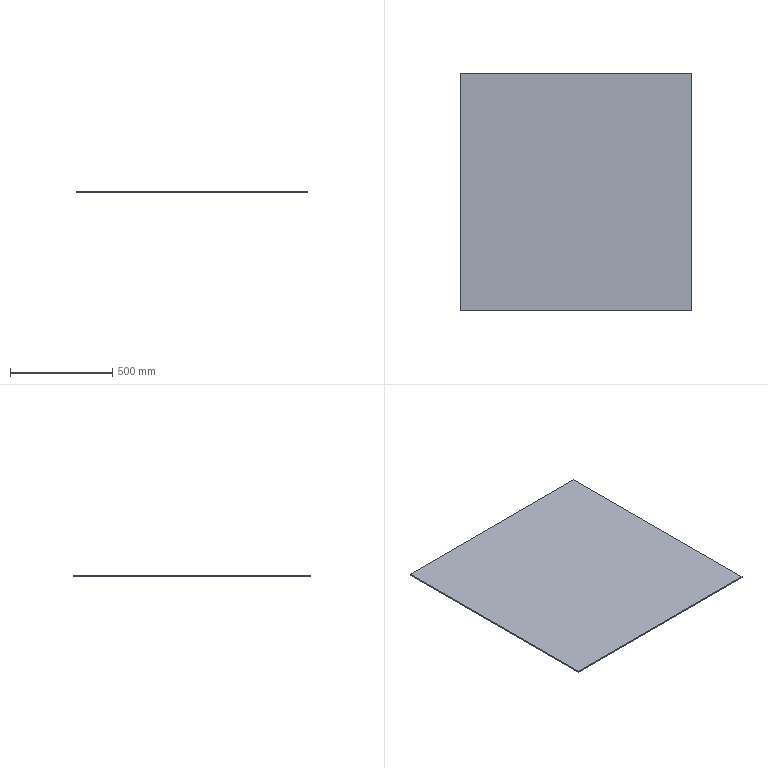Part | 1 solid | 6 faces | box 1135 x 1165 x 6 mm | volume 7933650 mm3 | plane 6
STEP:
#1=CARTESIAN_POINT('',(567.5,-582.5,0.));
#2=VERTEX_POINT('',#1);
#3=CARTESIAN_POINT('',(567.5,582.5,0.));
#4=VERTEX_POINT('',#3);
#5=CARTESIAN_POINT('',(567.5,582.5,0.));
#6=DIRECTION('',(0.,1.,0.));
#7=VECTOR('',#6,1000.);
#8=LINE('',#5,#7);
#9=EDGE_CURVE('',#2,#4,#8,.T.);
#10=ORIENTED_EDGE('',*,*,#9,.T.);
#11=CARTESIAN_POINT('',(567.5,582.5,6.));
#12=VERTEX_POINT('',#11);
#13=CARTESIAN_POINT('',(567.5,582.5,6.));
#14=DIRECTION('',(0.,0.,-1.));
#15=VECTOR('',#14,1000.);
#16=LINE('',#13,#15);
#17=EDGE_CURVE('',#12,#4,#16,.T.);
#18=ORIENTED_EDGE('',*,*,#17,.F.);
#19=CARTESIAN_POINT('',(567.5,-582.5,6.));
#20=VERTEX_POINT('',#19);
#21=CARTESIAN_POINT('',(567.5,582.5,6.));
#22=DIRECTION('',(0.,1.,0.));
#23=VECTOR('',#22,1000.);
#24=LINE('',#21,#23);
#25=EDGE_CURVE('',#20,#12,#24,.T.);
#26=ORIENTED_EDGE('',*,*,#25,.F.);
#27=CARTESIAN_POINT('',(567.5,-582.5,6.));
#28=DIRECTION('',(0.,0.,-1.));
#29=VECTOR('',#28,1000.);
#30=LINE('',#27,#29);
#31=EDGE_CURVE('',#20,#2,#30,.T.);
#32=ORIENTED_EDGE('',*,*,#31,.T.);
#33=EDGE_LOOP('',(#10,#18,#26,#32));
#34=FACE_OUTER_BOUND('',#33,.T.);
#35=CARTESIAN_POINT('',(567.5,582.5,6.));
#36=DIRECTION('',(-1.,0.,0.));
#37=DIRECTION('',(0.,-1.,0.));
#38=AXIS2_PLACEMENT_3D('',#35,#36,#37);
#39=PLANE('',#38);
#40=ADVANCED_FACE('',(#34),#39,.F.);
#41=CARTESIAN_POINT('',(-567.5,582.5,0.));
#42=VERTEX_POINT('',#41);
#43=CARTESIAN_POINT('',(-567.5,582.5,0.));
#44=DIRECTION('',(-1.,0.,0.));
#45=VECTOR('',#44,1000.);
#46=LINE('',#43,#45);
#47=EDGE_CURVE('',#4,#42,#46,.T.);
#48=ORIENTED_EDGE('',*,*,#47,.T.);
#49=CARTESIAN_POINT('',(-567.5,582.5,6.));
#50=VERTEX_POINT('',#49);
#51=CARTESIAN_POINT('',(-567.5,582.5,6.));
#52=DIRECTION('',(0.,0.,-1.));
#53=VECTOR('',#52,1000.);
#54=LINE('',#51,#53);
#55=EDGE_CURVE('',#50,#42,#54,.T.);
#56=ORIENTED_EDGE('',*,*,#55,.F.);
#57=CARTESIAN_POINT('',(-567.5,582.5,6.));
#58=DIRECTION('',(-1.,0.,0.));
#59=VECTOR('',#58,1000.);
#60=LINE('',#57,#59);
#61=EDGE_CURVE('',#12,#50,#60,.T.);
#62=ORIENTED_EDGE('',*,*,#61,.F.);
#63=ORIENTED_EDGE('',*,*,#17,.T.);
#64=EDGE_LOOP('',(#48,#56,#62,#63));
#65=FACE_OUTER_BOUND('',#64,.T.);
#66=CARTESIAN_POINT('',(-567.5,582.5,6.));
#67=DIRECTION('',(0.,-1.,0.));
#68=DIRECTION('',(0.,0.,-1.));
#69=AXIS2_PLACEMENT_3D('',#66,#67,#68);
#70=PLANE('',#69);
#71=ADVANCED_FACE('',(#65),#70,.F.);
#72=CARTESIAN_POINT('',(-567.5,-582.5,0.));
#73=VERTEX_POINT('',#72);
#74=CARTESIAN_POINT('',(-567.5,582.5,0.));
#75=DIRECTION('',(0.,-1.,0.));
#76=VECTOR('',#75,1000.);
#77=LINE('',#74,#76);
#78=EDGE_CURVE('',#42,#73,#77,.T.);
#79=ORIENTED_EDGE('',*,*,#78,.T.);
#80=CARTESIAN_POINT('',(-567.5,-582.5,6.));
#81=VERTEX_POINT('',#80);
#82=CARTESIAN_POINT('',(-567.5,-582.5,6.));
#83=DIRECTION('',(0.,0.,-1.));
#84=VECTOR('',#83,1000.);
#85=LINE('',#82,#84);
#86=EDGE_CURVE('',#81,#73,#85,.T.);
#87=ORIENTED_EDGE('',*,*,#86,.F.);
#88=CARTESIAN_POINT('',(-567.5,582.5,6.));
#89=DIRECTION('',(0.,-1.,0.));
#90=VECTOR('',#89,1000.);
#91=LINE('',#88,#90);
#92=EDGE_CURVE('',#50,#81,#91,.T.);
#93=ORIENTED_EDGE('',*,*,#92,.F.);
#94=ORIENTED_EDGE('',*,*,#55,.T.);
#95=EDGE_LOOP('',(#79,#87,#93,#94));
#96=FACE_OUTER_BOUND('',#95,.T.);
#97=CARTESIAN_POINT('',(-567.5,582.5,6.));
#98=DIRECTION('',(1.,0.,0.));
#99=DIRECTION('',(0.,1.,0.));
#100=AXIS2_PLACEMENT_3D('',#97,#98,#99);
#101=PLANE('',#100);
#102=ADVANCED_FACE('',(#96),#101,.F.);
#103=CARTESIAN_POINT('',(-567.5,-582.5,0.));
#104=DIRECTION('',(1.,0.,0.));
#105=VECTOR('',#104,1000.);
#106=LINE('',#103,#105);
#107=EDGE_CURVE('',#73,#2,#106,.T.);
#108=ORIENTED_EDGE('',*,*,#107,.T.);
#109=ORIENTED_EDGE('',*,*,#31,.F.);
#110=CARTESIAN_POINT('',(-567.5,-582.5,6.));
#111=DIRECTION('',(1.,0.,0.));
#112=VECTOR('',#111,1000.);
#113=LINE('',#110,#112);
#114=EDGE_CURVE('',#81,#20,#113,.T.);
#115=ORIENTED_EDGE('',*,*,#114,.F.);
#116=ORIENTED_EDGE('',*,*,#86,.T.);
#117=EDGE_LOOP('',(#108,#109,#115,#116));
#118=FACE_OUTER_BOUND('',#117,.T.);
#119=CARTESIAN_POINT('',(-567.5,-582.5,6.));
#120=DIRECTION('',(0.,1.,0.));
#121=DIRECTION('',(0.,0.,1.));
#122=AXIS2_PLACEMENT_3D('',#119,#120,#121);
#123=PLANE('',#122);
#124=ADVANCED_FACE('',(#118),#123,.F.);
#125=ORIENTED_EDGE('',*,*,#25,.T.);
#126=ORIENTED_EDGE('',*,*,#61,.T.);
#127=ORIENTED_EDGE('',*,*,#92,.T.);
#128=ORIENTED_EDGE('',*,*,#114,.T.);
#129=EDGE_LOOP('',(#125,#126,#127,#128));
#130=FACE_OUTER_BOUND('',#129,.T.);
#131=CARTESIAN_POINT('',(0.,0.,6.));
#132=DIRECTION('',(0.,0.,1.));
#133=DIRECTION('',(1.,0.,0.));
#134=AXIS2_PLACEMENT_3D('',#131,#132,#133);
#135=PLANE('',#134);
#136=ADVANCED_FACE('',(#130),#135,.T.);
#137=ORIENTED_EDGE('',*,*,#9,.F.);
#138=ORIENTED_EDGE('',*,*,#107,.F.);
#139=ORIENTED_EDGE('',*,*,#78,.F.);
#140=ORIENTED_EDGE('',*,*,#47,.F.);
#141=EDGE_LOOP('',(#137,#138,#139,#140));
#142=FACE_OUTER_BOUND('',#141,.T.);
#143=CARTESIAN_POINT('',(0.,0.,0.));
#144=DIRECTION('',(0.,0.,1.));
#145=DIRECTION('',(1.,0.,0.));
#146=AXIS2_PLACEMENT_3D('',#143,#144,#145);
#147=PLANE('',#146);
#148=ADVANCED_FACE('',(#142),#147,.F.);
#149=CLOSED_SHELL('',(#40,#71,#102,#124,#136,#148));
#150=MANIFOLD_SOLID_BREP('',#149);
#151=CARTESIAN_POINT('',(0.,0.,0.));
#152=DIRECTION('',(0.,0.,1.));
#153=DIRECTION('',(1.,0.,0.));
#154=AXIS2_PLACEMENT_3D('',#151,#152,#153);
#155=(LENGTH_UNIT()NAMED_UNIT(*)SI_UNIT(.MILLI.,.METRE.));
#156=UNCERTAINTY_MEASURE_WITH_UNIT(LENGTH_MEASURE(0.00001),#155,'','');
#157=(NAMED_UNIT(*)PLANE_ANGLE_UNIT()SI_UNIT($,.RADIAN.));
#158=(NAMED_UNIT(*)SI_UNIT($,.STERADIAN.)SOLID_ANGLE_UNIT());
#159=(GEOMETRIC_REPRESENTATION_CONTEXT(3)GLOBAL_UNCERTAINTY_ASSIGNED_CONTEXT((#156))GLOBAL_UNIT_ASSIGNED_CONTEXT((#155,#157,#158))REPRESENTATION_CONTEXT('',''));
#160=ADVANCED_BREP_SHAPE_REPRESENTATION('',(#150,#154),#159);